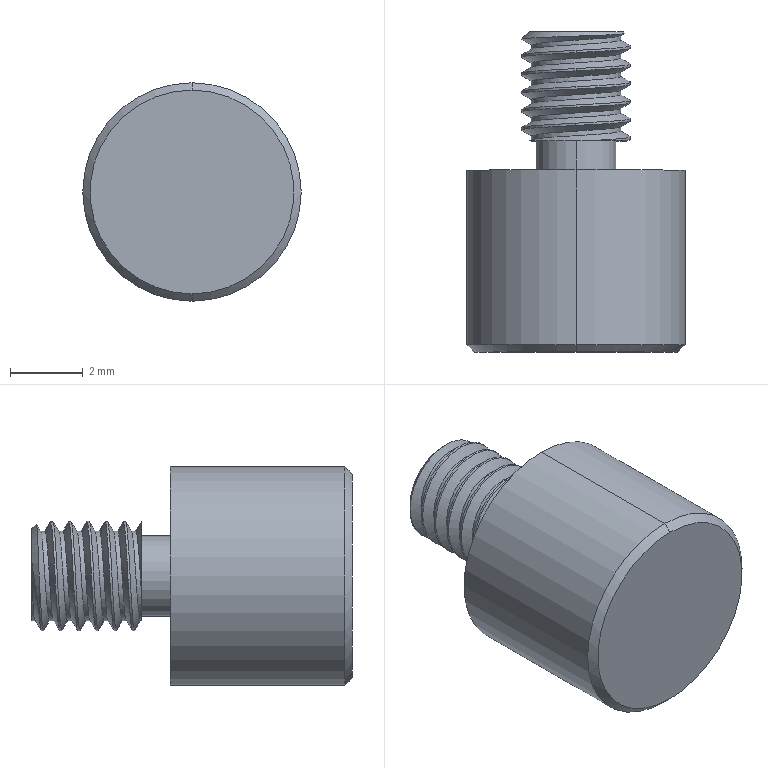Part | STEP file | 1 solid | 26 faces | box 6 x 8.8 x 6 mm | volume 161.192 mm3 | cylinder 16 | plane 4 | cone 3 | spline 3 | commonest cylinder face diameters 3 x12 2.2 x2 6 x2